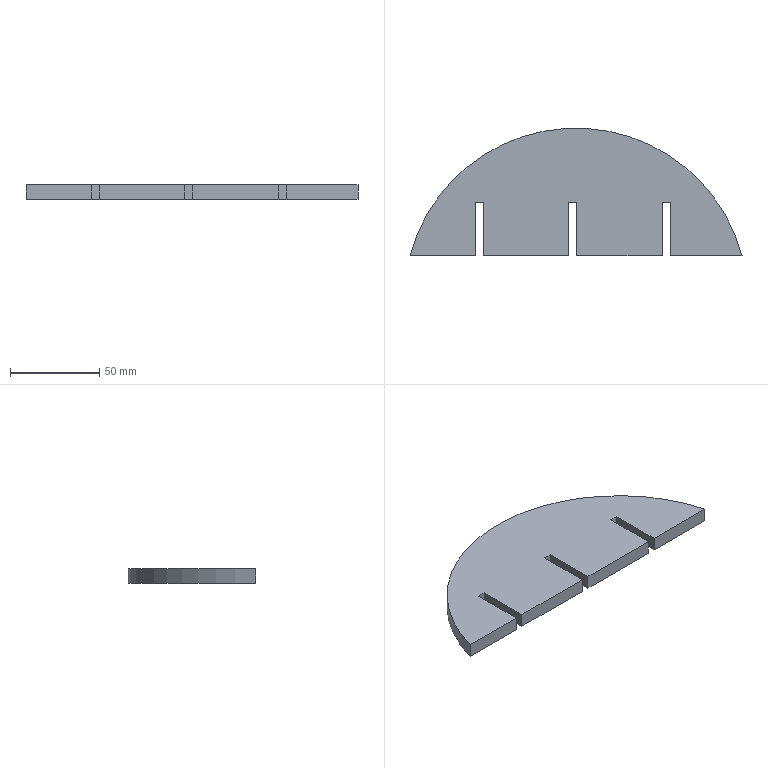Part | SolidWorks | features ICE 2, Extrusion 1 | 1 solid | 16 faces | box 186.411 x 71.5 x 8 mm | volume 75617 mm3 | plane 15 | cylinder 1 | commonest cylinder face diameters 193 x1
STEP:
#1=CARTESIAN_POINT('',(-54.75,25.,0.));
#2=VERTEX_POINT('',#1);
#3=CARTESIAN_POINT('',(-91.355,25.,0.));
#4=VERTEX_POINT('',#3);
#5=CARTESIAN_POINT('',(1.85,25.,0.));
#6=DIRECTION('',(-1.,0.,0.));
#7=VECTOR('',#6,1000.);
#8=LINE('',#5,#7);
#9=EDGE_CURVE('',#2,#4,#8,.T.);
#10=ORIENTED_EDGE('',*,*,#9,.F.);
#11=CARTESIAN_POINT('',(-54.75,25.,8.));
#12=VERTEX_POINT('',#11);
#13=CARTESIAN_POINT('',(-54.75,25.,10.));
#14=DIRECTION('',(0.,0.,-1.));
#15=VECTOR('',#14,1000.);
#16=LINE('',#13,#15);
#17=EDGE_CURVE('',#12,#2,#16,.T.);
#18=ORIENTED_EDGE('',*,*,#17,.F.);
#19=CARTESIAN_POINT('',(-91.355,25.,8.));
#20=VERTEX_POINT('',#19);
#21=CARTESIAN_POINT('',(-94.65,25.,8.));
#22=DIRECTION('',(-1.,0.,0.));
#23=VECTOR('',#22,1000.);
#24=LINE('',#21,#23);
#25=EDGE_CURVE('',#12,#20,#24,.T.);
#26=ORIENTED_EDGE('',*,*,#25,.T.);
#27=CARTESIAN_POINT('',(-91.355,25.,8.));
#28=DIRECTION('',(0.,0.,1.));
#29=VECTOR('',#28,1000.);
#30=LINE('',#27,#29);
#31=EDGE_CURVE('',#4,#20,#30,.T.);
#32=ORIENTED_EDGE('',*,*,#31,.F.);
#33=EDGE_LOOP('',(#10,#18,#26,#32));
#34=FACE_OUTER_BOUND('',#33,.T.);
#35=CARTESIAN_POINT('',(-94.65,25.,-2.));
#36=DIRECTION('',(0.,1.,0.));
#37=DIRECTION('',(0.,0.,1.));
#38=AXIS2_PLACEMENT_3D('',#35,#36,#37);
#39=PLANE('',#38);
#40=ADVANCED_FACE('',(#34),#39,.F.);
#41=CARTESIAN_POINT('',(-2.25,25.,8.));
#42=VERTEX_POINT('',#41);
#43=CARTESIAN_POINT('',(-50.25,25.,8.));
#44=VERTEX_POINT('',#43);
#45=CARTESIAN_POINT('',(-94.65,25.,8.));
#46=DIRECTION('',(-1.,0.,0.));
#47=VECTOR('',#46,1000.);
#48=LINE('',#45,#47);
#49=EDGE_CURVE('',#42,#44,#48,.T.);
#50=ORIENTED_EDGE('',*,*,#49,.T.);
#51=CARTESIAN_POINT('',(-50.25,25.,0.));
#52=VERTEX_POINT('',#51);
#53=CARTESIAN_POINT('',(-50.25,25.,10.));
#54=DIRECTION('',(0.,0.,-1.));
#55=VECTOR('',#54,1000.);
#56=LINE('',#53,#55);
#57=EDGE_CURVE('',#44,#52,#56,.T.);
#58=ORIENTED_EDGE('',*,*,#57,.T.);
#59=CARTESIAN_POINT('',(-2.25,25.,0.));
#60=VERTEX_POINT('',#59);
#61=CARTESIAN_POINT('',(1.85,25.,0.));
#62=DIRECTION('',(-1.,0.,0.));
#63=VECTOR('',#62,1000.);
#64=LINE('',#61,#63);
#65=EDGE_CURVE('',#60,#52,#64,.T.);
#66=ORIENTED_EDGE('',*,*,#65,.F.);
#67=CARTESIAN_POINT('',(-2.25,25.,10.));
#68=DIRECTION('',(0.,0.,-1.));
#69=VECTOR('',#68,1000.);
#70=LINE('',#67,#69);
#71=EDGE_CURVE('',#42,#60,#70,.T.);
#72=ORIENTED_EDGE('',*,*,#71,.F.);
#73=EDGE_LOOP('',(#50,#58,#66,#72));
#74=FACE_OUTER_BOUND('',#73,.T.);
#75=CARTESIAN_POINT('',(-94.65,25.,-2.));
#76=DIRECTION('',(0.,1.,0.));
#77=DIRECTION('',(0.,0.,1.));
#78=AXIS2_PLACEMENT_3D('',#75,#76,#77);
#79=PLANE('',#78);
#80=ADVANCED_FACE('',(#74),#79,.F.);
#81=CARTESIAN_POINT('',(50.25,25.,8.));
#82=VERTEX_POINT('',#81);
#83=CARTESIAN_POINT('',(2.25,25.,8.));
#84=VERTEX_POINT('',#83);
#85=CARTESIAN_POINT('',(-94.65,25.,8.));
#86=DIRECTION('',(-1.,0.,0.));
#87=VECTOR('',#86,1000.);
#88=LINE('',#85,#87);
#89=EDGE_CURVE('',#82,#84,#88,.T.);
#90=ORIENTED_EDGE('',*,*,#89,.T.);
#91=CARTESIAN_POINT('',(2.25,25.,0.));
#92=VERTEX_POINT('',#91);
#93=CARTESIAN_POINT('',(2.25,25.,10.));
#94=DIRECTION('',(0.,0.,-1.));
#95=VECTOR('',#94,1000.);
#96=LINE('',#93,#95);
#97=EDGE_CURVE('',#84,#92,#96,.T.);
#98=ORIENTED_EDGE('',*,*,#97,.T.);
#99=CARTESIAN_POINT('',(50.25,25.,0.));
#100=VERTEX_POINT('',#99);
#101=CARTESIAN_POINT('',(1.85,25.,0.));
#102=DIRECTION('',(-1.,0.,0.));
#103=VECTOR('',#102,1000.);
#104=LINE('',#101,#103);
#105=EDGE_CURVE('',#100,#92,#104,.T.);
#106=ORIENTED_EDGE('',*,*,#105,.F.);
#107=CARTESIAN_POINT('',(50.25,25.,-2.));
#108=DIRECTION('',(0.,0.,1.));
#109=VECTOR('',#108,1000.);
#110=LINE('',#107,#109);
#111=EDGE_CURVE('',#100,#82,#110,.T.);
#112=ORIENTED_EDGE('',*,*,#111,.T.);
#113=EDGE_LOOP('',(#90,#98,#106,#112));
#114=FACE_OUTER_BOUND('',#113,.T.);
#115=CARTESIAN_POINT('',(-94.65,25.,-2.));
#116=DIRECTION('',(0.,1.,0.));
#117=DIRECTION('',(0.,0.,1.));
#118=AXIS2_PLACEMENT_3D('',#115,#116,#117);
#119=PLANE('',#118);
#120=ADVANCED_FACE('',(#114),#119,.F.);
#121=CARTESIAN_POINT('',(95.055,25.,8.));
#122=VERTEX_POINT('',#121);
#123=CARTESIAN_POINT('',(1.85,0.,8.));
#124=DIRECTION('',(0.,0.,1.));
#125=DIRECTION('',(1.,0.,0.));
#126=AXIS2_PLACEMENT_3D('',#123,#124,#125);
#127=CIRCLE('',#126,96.5);
#128=EDGE_CURVE('',#122,#20,#127,.T.);
#129=ORIENTED_EDGE('',*,*,#128,.F.);
#130=CARTESIAN_POINT('',(95.055,25.,0.));
#131=VERTEX_POINT('',#130);
#132=CARTESIAN_POINT('',(95.055,25.,8.));
#133=DIRECTION('',(0.,0.,-1.));
#134=VECTOR('',#133,1000.);
#135=LINE('',#132,#134);
#136=EDGE_CURVE('',#122,#131,#135,.T.);
#137=ORIENTED_EDGE('',*,*,#136,.T.);
#138=CARTESIAN_POINT('',(1.85,0.,0.));
#139=DIRECTION('',(0.,0.,1.));
#140=DIRECTION('',(1.,0.,0.));
#141=AXIS2_PLACEMENT_3D('',#138,#139,#140);
#142=CIRCLE('',#141,96.5);
#143=EDGE_CURVE('',#131,#4,#142,.T.);
#144=ORIENTED_EDGE('',*,*,#143,.T.);
#145=ORIENTED_EDGE('',*,*,#31,.T.);
#146=EDGE_LOOP('',(#129,#137,#144,#145));
#147=FACE_OUTER_BOUND('',#146,.T.);
#148=CARTESIAN_POINT('',(1.85,0.,8.));
#149=DIRECTION('',(0.,0.,-1.));
#150=DIRECTION('',(-1.,0.,0.));
#151=AXIS2_PLACEMENT_3D('',#148,#149,#150);
#152=CYLINDRICAL_SURFACE('',#151,96.5);
#153=ADVANCED_FACE('',(#147),#152,.T.);
#154=CARTESIAN_POINT('',(-54.75,55.,8.));
#155=VERTEX_POINT('',#154);
#156=CARTESIAN_POINT('',(-54.75,0.,8.));
#157=DIRECTION('',(0.,-1.,0.));
#158=VECTOR('',#157,1000.);
#159=LINE('',#156,#158);
#160=EDGE_CURVE('',#155,#12,#159,.T.);
#161=ORIENTED_EDGE('',*,*,#160,.F.);
#162=CARTESIAN_POINT('',(-50.25,55.,8.));
#163=VERTEX_POINT('',#162);
#164=CARTESIAN_POINT('',(1.85,55.,8.));
#165=DIRECTION('',(-1.,0.,0.));
#166=VECTOR('',#165,1000.);
#167=LINE('',#164,#166);
#168=EDGE_CURVE('',#163,#155,#167,.T.);
#169=ORIENTED_EDGE('',*,*,#168,.F.);
#170=CARTESIAN_POINT('',(-50.25,0.,8.));
#171=DIRECTION('',(0.,1.,0.));
#172=VECTOR('',#171,1000.);
#173=LINE('',#170,#172);
#174=EDGE_CURVE('',#44,#163,#173,.T.);
#175=ORIENTED_EDGE('',*,*,#174,.F.);
#176=ORIENTED_EDGE('',*,*,#49,.F.);
#177=CARTESIAN_POINT('',(-2.25,55.,8.));
#178=VERTEX_POINT('',#177);
#179=CARTESIAN_POINT('',(-2.25,0.,8.));
#180=DIRECTION('',(0.,-1.,0.));
#181=VECTOR('',#180,1000.);
#182=LINE('',#179,#181);
#183=EDGE_CURVE('',#178,#42,#182,.T.);
#184=ORIENTED_EDGE('',*,*,#183,.F.);
#185=CARTESIAN_POINT('',(2.25,55.,8.));
#186=VERTEX_POINT('',#185);
#187=CARTESIAN_POINT('',(1.85,55.,8.));
#188=DIRECTION('',(-1.,0.,0.));
#189=VECTOR('',#188,1000.);
#190=LINE('',#187,#189);
#191=EDGE_CURVE('',#186,#178,#190,.T.);
#192=ORIENTED_EDGE('',*,*,#191,.F.);
#193=CARTESIAN_POINT('',(2.25,0.,8.));
#194=DIRECTION('',(0.,1.,0.));
#195=VECTOR('',#194,1000.);
#196=LINE('',#193,#195);
#197=EDGE_CURVE('',#84,#186,#196,.T.);
#198=ORIENTED_EDGE('',*,*,#197,.F.);
#199=ORIENTED_EDGE('',*,*,#89,.F.);
#200=CARTESIAN_POINT('',(50.25,55.,8.));
#201=VERTEX_POINT('',#200);
#202=CARTESIAN_POINT('',(50.25,0.,8.));
#203=DIRECTION('',(0.,-1.,0.));
#204=VECTOR('',#203,1000.);
#205=LINE('',#202,#204);
#206=EDGE_CURVE('',#201,#82,#205,.T.);
#207=ORIENTED_EDGE('',*,*,#206,.F.);
#208=CARTESIAN_POINT('',(54.75,55.,8.));
#209=VERTEX_POINT('',#208);
#210=CARTESIAN_POINT('',(1.85,55.,8.));
#211=DIRECTION('',(-1.,0.,0.));
#212=VECTOR('',#211,1000.);
#213=LINE('',#210,#212);
#214=EDGE_CURVE('',#209,#201,#213,.T.);
#215=ORIENTED_EDGE('',*,*,#214,.F.);
#216=CARTESIAN_POINT('',(54.75,25.,8.));
#217=VERTEX_POINT('',#216);
#218=CARTESIAN_POINT('',(54.75,0.,8.));
#219=DIRECTION('',(0.,1.,0.));
#220=VECTOR('',#219,1000.);
#221=LINE('',#218,#220);
#222=EDGE_CURVE('',#217,#209,#221,.T.);
#223=ORIENTED_EDGE('',*,*,#222,.F.);
#224=CARTESIAN_POINT('',(-94.65,25.,8.));
#225=DIRECTION('',(-1.,0.,0.));
#226=VECTOR('',#225,1000.);
#227=LINE('',#224,#226);
#228=EDGE_CURVE('',#122,#217,#227,.T.);
#229=ORIENTED_EDGE('',*,*,#228,.F.);
#230=ORIENTED_EDGE('',*,*,#128,.T.);
#231=ORIENTED_EDGE('',*,*,#25,.F.);
#232=EDGE_LOOP('',(#161,#169,#175,#176,#184,#192,#198,#199,#207,#215,#223,#229,#230,#231));
#233=FACE_OUTER_BOUND('',#232,.T.);
#234=CARTESIAN_POINT('',(1.85,0.,8.));
#235=DIRECTION('',(0.,0.,1.));
#236=DIRECTION('',(1.,0.,0.));
#237=AXIS2_PLACEMENT_3D('',#234,#235,#236);
#238=PLANE('',#237);
#239=ADVANCED_FACE('',(#233),#238,.T.);
#240=CARTESIAN_POINT('',(-54.75,55.,0.));
#241=VERTEX_POINT('',#240);
#242=CARTESIAN_POINT('',(-50.25,55.,0.));
#243=VERTEX_POINT('',#242);
#244=CARTESIAN_POINT('',(-54.75,55.,0.));
#245=DIRECTION('',(1.,0.,0.));
#246=VECTOR('',#245,1000.);
#247=LINE('',#244,#246);
#248=EDGE_CURVE('',#241,#243,#247,.T.);
#249=ORIENTED_EDGE('',*,*,#248,.F.);
#250=CARTESIAN_POINT('',(-54.75,25.,0.));
#251=DIRECTION('',(0.,1.,0.));
#252=VECTOR('',#251,1000.);
#253=LINE('',#250,#252);
#254=EDGE_CURVE('',#2,#241,#253,.T.);
#255=ORIENTED_EDGE('',*,*,#254,.F.);
#256=ORIENTED_EDGE('',*,*,#9,.T.);
#257=ORIENTED_EDGE('',*,*,#143,.F.);
#258=CARTESIAN_POINT('',(54.75,25.,0.));
#259=VERTEX_POINT('',#258);
#260=CARTESIAN_POINT('',(1.85,25.,0.));
#261=DIRECTION('',(-1.,0.,0.));
#262=VECTOR('',#261,1000.);
#263=LINE('',#260,#262);
#264=EDGE_CURVE('',#131,#259,#263,.T.);
#265=ORIENTED_EDGE('',*,*,#264,.T.);
#266=CARTESIAN_POINT('',(54.75,55.,0.));
#267=VERTEX_POINT('',#266);
#268=CARTESIAN_POINT('',(54.75,25.,0.));
#269=DIRECTION('',(0.,-1.,0.));
#270=VECTOR('',#269,1000.);
#271=LINE('',#268,#270);
#272=EDGE_CURVE('',#267,#259,#271,.T.);
#273=ORIENTED_EDGE('',*,*,#272,.F.);
#274=CARTESIAN_POINT('',(50.25,55.,0.));
#275=VERTEX_POINT('',#274);
#276=CARTESIAN_POINT('',(50.25,55.,0.));
#277=DIRECTION('',(1.,0.,0.));
#278=VECTOR('',#277,1000.);
#279=LINE('',#276,#278);
#280=EDGE_CURVE('',#275,#267,#279,.T.);
#281=ORIENTED_EDGE('',*,*,#280,.F.);
#282=CARTESIAN_POINT('',(50.25,25.,0.));
#283=DIRECTION('',(0.,1.,0.));
#284=VECTOR('',#283,1000.);
#285=LINE('',#282,#284);
#286=EDGE_CURVE('',#100,#275,#285,.T.);
#287=ORIENTED_EDGE('',*,*,#286,.F.);
#288=ORIENTED_EDGE('',*,*,#105,.T.);
#289=CARTESIAN_POINT('',(2.25,55.,0.));
#290=VERTEX_POINT('',#289);
#291=CARTESIAN_POINT('',(2.25,55.,0.));
#292=DIRECTION('',(0.,-1.,0.));
#293=VECTOR('',#292,1000.);
#294=LINE('',#291,#293);
#295=EDGE_CURVE('',#290,#92,#294,.T.);
#296=ORIENTED_EDGE('',*,*,#295,.F.);
#297=CARTESIAN_POINT('',(-2.25,55.,0.));
#298=VERTEX_POINT('',#297);
#299=CARTESIAN_POINT('',(2.25,55.,0.));
#300=DIRECTION('',(1.,0.,0.));
#301=VECTOR('',#300,1000.);
#302=LINE('',#299,#301);
#303=EDGE_CURVE('',#298,#290,#302,.T.);
#304=ORIENTED_EDGE('',*,*,#303,.F.);
#305=CARTESIAN_POINT('',(-2.25,25.,0.));
#306=DIRECTION('',(0.,1.,0.));
#307=VECTOR('',#306,1000.);
#308=LINE('',#305,#307);
#309=EDGE_CURVE('',#60,#298,#308,.T.);
#310=ORIENTED_EDGE('',*,*,#309,.F.);
#311=ORIENTED_EDGE('',*,*,#65,.T.);
#312=CARTESIAN_POINT('',(-50.25,25.,0.));
#313=DIRECTION('',(0.,-1.,0.));
#314=VECTOR('',#313,1000.);
#315=LINE('',#312,#314);
#316=EDGE_CURVE('',#243,#52,#315,.T.);
#317=ORIENTED_EDGE('',*,*,#316,.F.);
#318=EDGE_LOOP('',(#249,#255,#256,#257,#265,#273,#281,#287,#288,#296,#304,#310,#311,#317));
#319=FACE_OUTER_BOUND('',#318,.T.);
#320=CARTESIAN_POINT('',(1.85,0.,0.));
#321=DIRECTION('',(0.,0.,1.));
#322=DIRECTION('',(1.,0.,0.));
#323=AXIS2_PLACEMENT_3D('',#320,#321,#322);
#324=PLANE('',#323);
#325=ADVANCED_FACE('',(#319),#324,.F.);
#326=ORIENTED_EDGE('',*,*,#228,.T.);
#327=CARTESIAN_POINT('',(54.75,25.,-2.));
#328=DIRECTION('',(0.,0.,-1.));
#329=VECTOR('',#328,1000.);
#330=LINE('',#327,#329);
#331=EDGE_CURVE('',#217,#259,#330,.T.);
#332=ORIENTED_EDGE('',*,*,#331,.T.);
#333=ORIENTED_EDGE('',*,*,#264,.F.);
#334=ORIENTED_EDGE('',*,*,#136,.F.);
#335=EDGE_LOOP('',(#326,#332,#333,#334));
#336=FACE_OUTER_BOUND('',#335,.T.);
#337=CARTESIAN_POINT('',(-94.65,25.,-2.));
#338=DIRECTION('',(0.,1.,0.));
#339=DIRECTION('',(0.,0.,1.));
#340=AXIS2_PLACEMENT_3D('',#337,#338,#339);
#341=PLANE('',#340);
#342=ADVANCED_FACE('',(#336),#341,.F.);
#343=ORIENTED_EDGE('',*,*,#206,.T.);
#344=ORIENTED_EDGE('',*,*,#111,.F.);
#345=ORIENTED_EDGE('',*,*,#286,.T.);
#346=CARTESIAN_POINT('',(50.25,55.,10.));
#347=DIRECTION('',(0.,0.,-1.));
#348=VECTOR('',#347,1000.);
#349=LINE('',#346,#348);
#350=EDGE_CURVE('',#201,#275,#349,.T.);
#351=ORIENTED_EDGE('',*,*,#350,.F.);
#352=EDGE_LOOP('',(#343,#344,#345,#351));
#353=FACE_OUTER_BOUND('',#352,.T.);
#354=CARTESIAN_POINT('',(50.25,25.,10.));
#355=DIRECTION('',(-1.,0.,0.));
#356=DIRECTION('',(0.,0.,1.));
#357=AXIS2_PLACEMENT_3D('',#354,#355,#356);
#358=PLANE('',#357);
#359=ADVANCED_FACE('',(#353),#358,.F.);
#360=ORIENTED_EDGE('',*,*,#222,.T.);
#361=CARTESIAN_POINT('',(54.75,55.,10.));
#362=DIRECTION('',(0.,0.,-1.));
#363=VECTOR('',#362,1000.);
#364=LINE('',#361,#363);
#365=EDGE_CURVE('',#209,#267,#364,.T.);
#366=ORIENTED_EDGE('',*,*,#365,.T.);
#367=ORIENTED_EDGE('',*,*,#272,.T.);
#368=ORIENTED_EDGE('',*,*,#331,.F.);
#369=EDGE_LOOP('',(#360,#366,#367,#368));
#370=FACE_OUTER_BOUND('',#369,.T.);
#371=CARTESIAN_POINT('',(54.75,25.,10.));
#372=DIRECTION('',(1.,0.,0.));
#373=DIRECTION('',(0.,0.,-1.));
#374=AXIS2_PLACEMENT_3D('',#371,#372,#373);
#375=PLANE('',#374);
#376=ADVANCED_FACE('',(#370),#375,.F.);
#377=ORIENTED_EDGE('',*,*,#214,.T.);
#378=ORIENTED_EDGE('',*,*,#350,.T.);
#379=ORIENTED_EDGE('',*,*,#280,.T.);
#380=ORIENTED_EDGE('',*,*,#365,.F.);
#381=EDGE_LOOP('',(#377,#378,#379,#380));
#382=FACE_OUTER_BOUND('',#381,.T.);
#383=CARTESIAN_POINT('',(50.25,55.,10.));
#384=DIRECTION('',(0.,1.,0.));
#385=DIRECTION('',(0.,0.,1.));
#386=AXIS2_PLACEMENT_3D('',#383,#384,#385);
#387=PLANE('',#386);
#388=ADVANCED_FACE('',(#382),#387,.F.);
#389=ORIENTED_EDGE('',*,*,#183,.T.);
#390=ORIENTED_EDGE('',*,*,#71,.T.);
#391=ORIENTED_EDGE('',*,*,#309,.T.);
#392=CARTESIAN_POINT('',(-2.25,55.,10.));
#393=DIRECTION('',(0.,0.,-1.));
#394=VECTOR('',#393,1000.);
#395=LINE('',#392,#394);
#396=EDGE_CURVE('',#178,#298,#395,.T.);
#397=ORIENTED_EDGE('',*,*,#396,.F.);
#398=EDGE_LOOP('',(#389,#390,#391,#397));
#399=FACE_OUTER_BOUND('',#398,.T.);
#400=CARTESIAN_POINT('',(-2.25,25.,10.));
#401=DIRECTION('',(-1.,0.,0.));
#402=DIRECTION('',(0.,-1.,0.));
#403=AXIS2_PLACEMENT_3D('',#400,#401,#402);
#404=PLANE('',#403);
#405=ADVANCED_FACE('',(#399),#404,.F.);
#406=ORIENTED_EDGE('',*,*,#197,.T.);
#407=CARTESIAN_POINT('',(2.25,55.,10.));
#408=DIRECTION('',(0.,0.,-1.));
#409=VECTOR('',#408,1000.);
#410=LINE('',#407,#409);
#411=EDGE_CURVE('',#186,#290,#410,.T.);
#412=ORIENTED_EDGE('',*,*,#411,.T.);
#413=ORIENTED_EDGE('',*,*,#295,.T.);
#414=ORIENTED_EDGE('',*,*,#97,.F.);
#415=EDGE_LOOP('',(#406,#412,#413,#414));
#416=FACE_OUTER_BOUND('',#415,.T.);
#417=CARTESIAN_POINT('',(2.25,55.,10.));
#418=DIRECTION('',(1.,0.,0.));
#419=DIRECTION('',(0.,1.,0.));
#420=AXIS2_PLACEMENT_3D('',#417,#418,#419);
#421=PLANE('',#420);
#422=ADVANCED_FACE('',(#416),#421,.F.);
#423=ORIENTED_EDGE('',*,*,#191,.T.);
#424=ORIENTED_EDGE('',*,*,#396,.T.);
#425=ORIENTED_EDGE('',*,*,#303,.T.);
#426=ORIENTED_EDGE('',*,*,#411,.F.);
#427=EDGE_LOOP('',(#423,#424,#425,#426));
#428=FACE_OUTER_BOUND('',#427,.T.);
#429=CARTESIAN_POINT('',(2.25,55.,10.));
#430=DIRECTION('',(0.,1.,0.));
#431=DIRECTION('',(0.,0.,1.));
#432=AXIS2_PLACEMENT_3D('',#429,#430,#431);
#433=PLANE('',#432);
#434=ADVANCED_FACE('',(#428),#433,.F.);
#435=ORIENTED_EDGE('',*,*,#160,.T.);
#436=ORIENTED_EDGE('',*,*,#17,.T.);
#437=ORIENTED_EDGE('',*,*,#254,.T.);
#438=CARTESIAN_POINT('',(-54.75,55.,10.));
#439=DIRECTION('',(0.,0.,-1.));
#440=VECTOR('',#439,1000.);
#441=LINE('',#438,#440);
#442=EDGE_CURVE('',#155,#241,#441,.T.);
#443=ORIENTED_EDGE('',*,*,#442,.F.);
#444=EDGE_LOOP('',(#435,#436,#437,#443));
#445=FACE_OUTER_BOUND('',#444,.T.);
#446=CARTESIAN_POINT('',(-54.75,25.,10.));
#447=DIRECTION('',(-1.,0.,0.));
#448=DIRECTION('',(0.,0.,1.));
#449=AXIS2_PLACEMENT_3D('',#446,#447,#448);
#450=PLANE('',#449);
#451=ADVANCED_FACE('',(#445),#450,.F.);
#452=ORIENTED_EDGE('',*,*,#174,.T.);
#453=CARTESIAN_POINT('',(-50.25,55.,10.));
#454=DIRECTION('',(0.,0.,-1.));
#455=VECTOR('',#454,1000.);
#456=LINE('',#453,#455);
#457=EDGE_CURVE('',#163,#243,#456,.T.);
#458=ORIENTED_EDGE('',*,*,#457,.T.);
#459=ORIENTED_EDGE('',*,*,#316,.T.);
#460=ORIENTED_EDGE('',*,*,#57,.F.);
#461=EDGE_LOOP('',(#452,#458,#459,#460));
#462=FACE_OUTER_BOUND('',#461,.T.);
#463=CARTESIAN_POINT('',(-50.25,25.,10.));
#464=DIRECTION('',(1.,0.,0.));
#465=DIRECTION('',(0.,0.,-1.));
#466=AXIS2_PLACEMENT_3D('',#463,#464,#465);
#467=PLANE('',#466);
#468=ADVANCED_FACE('',(#462),#467,.F.);
#469=ORIENTED_EDGE('',*,*,#168,.T.);
#470=ORIENTED_EDGE('',*,*,#442,.T.);
#471=ORIENTED_EDGE('',*,*,#248,.T.);
#472=ORIENTED_EDGE('',*,*,#457,.F.);
#473=EDGE_LOOP('',(#469,#470,#471,#472));
#474=FACE_OUTER_BOUND('',#473,.T.);
#475=CARTESIAN_POINT('',(-54.75,55.,10.));
#476=DIRECTION('',(0.,1.,0.));
#477=DIRECTION('',(0.,0.,1.));
#478=AXIS2_PLACEMENT_3D('',#475,#476,#477);
#479=PLANE('',#478);
#480=ADVANCED_FACE('',(#474),#479,.F.);
#481=CLOSED_SHELL('',(#40,#80,#120,#153,#239,#325,#342,#359,#376,#388,#405,#422,#434,#451,#468,#480));
#482=MANIFOLD_SOLID_BREP('',#481);
#483=CARTESIAN_POINT('',(0.,0.,0.));
#484=DIRECTION('',(0.,0.,1.));
#485=DIRECTION('',(1.,0.,0.));
#486=AXIS2_PLACEMENT_3D('',#483,#484,#485);
#487=(LENGTH_UNIT()NAMED_UNIT(*)SI_UNIT(.MILLI.,.METRE.));
#488=UNCERTAINTY_MEASURE_WITH_UNIT(LENGTH_MEASURE(0.00001),#487,'','');
#489=(NAMED_UNIT(*)PLANE_ANGLE_UNIT()SI_UNIT($,.RADIAN.));
#490=(NAMED_UNIT(*)SI_UNIT($,.STERADIAN.)SOLID_ANGLE_UNIT());
#491=(GEOMETRIC_REPRESENTATION_CONTEXT(3)GLOBAL_UNCERTAINTY_ASSIGNED_CONTEXT((#488))GLOBAL_UNIT_ASSIGNED_CONTEXT((#487,#489,#490))REPRESENTATION_CONTEXT('',''));
#492=ADVANCED_BREP_SHAPE_REPRESENTATION('',(#482,#486),#491);